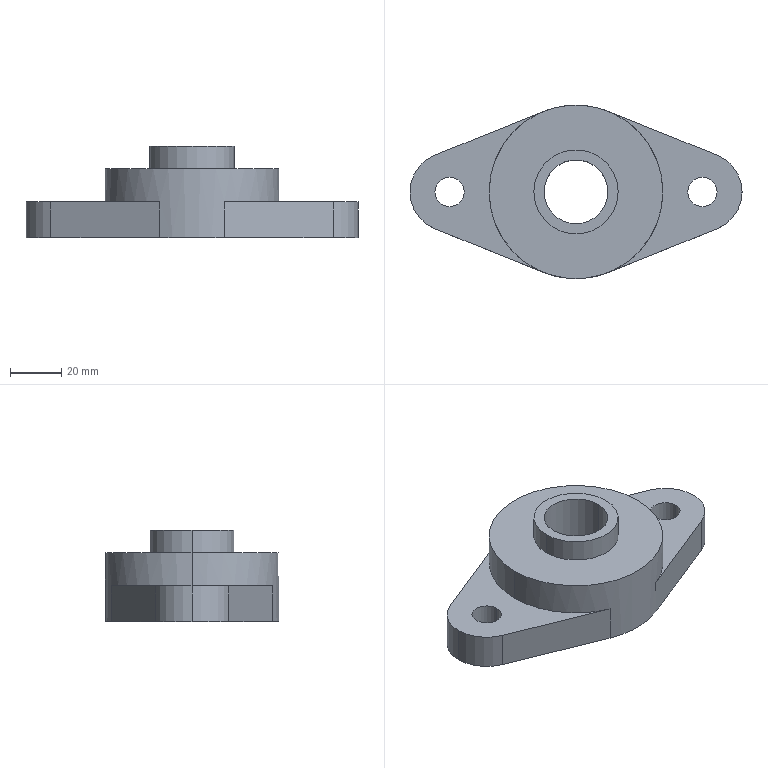Part | STEP file | UCFL205 | 1 solid | 27 faces | box 130 x 68 x 35.7 mm | volume 116034 mm3 | cylinder 15 | plane 10 | torus 2 | commonest cylinder face diameters 11.5 x4 31 x3 25 x2 33 x2 48 x2 68 x2